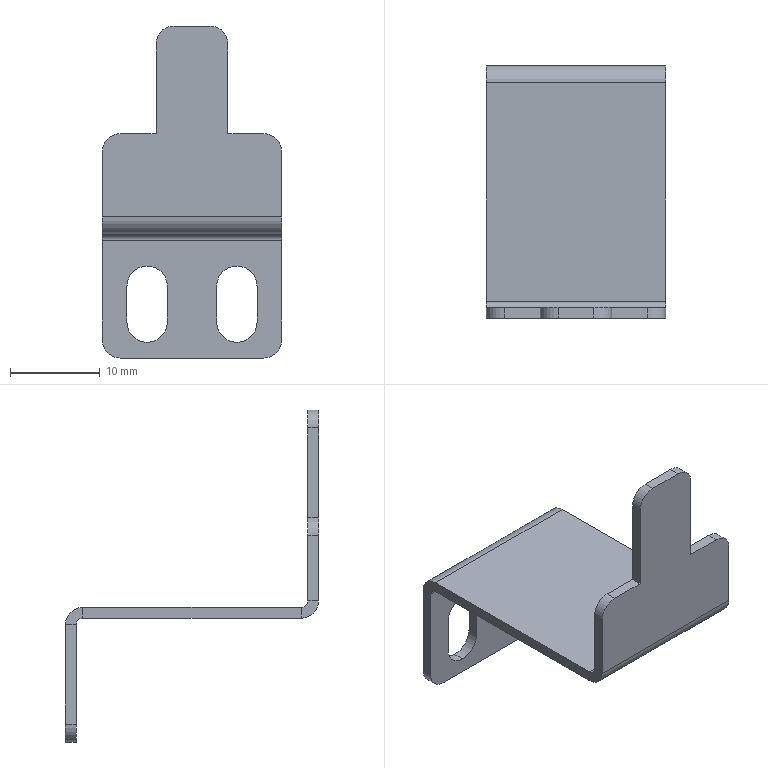Part | SolidWorks | features Cut 1, Fillet 1, FlatPattern 1, HoleWzd 1, SMBaseFlange 1, SheetMetal 1 | 1 solid | 42 faces | box 20 x 28.2 x 37 mm | volume 1248 mm3 | plane 26 | cylinder 16 | commonest cylinder face diameters 4 x6 4.5 x6 1.473 x2 3.873 x2
STEP:
#1=CARTESIAN_POINT('',(17.25,27.,-33.));
#2=VERTEX_POINT('',#1);
#3=CARTESIAN_POINT('',(15.,27.,-35.25));
#4=VERTEX_POINT('',#3);
#5=CARTESIAN_POINT('',(15.,27.,-33.));
#6=DIRECTION('',(0.,1.,0.));
#7=DIRECTION('',(0.,0.,1.));
#8=AXIS2_PLACEMENT_3D('',#5,#6,#7);
#9=CIRCLE('',#8,2.25);
#10=EDGE_CURVE('',#2,#4,#9,.T.);
#11=ORIENTED_EDGE('',*,*,#10,.T.);
#12=CARTESIAN_POINT('',(15.,25.8,-35.25));
#13=VERTEX_POINT('',#12);
#14=CARTESIAN_POINT('',(15.,25.8,-35.25));
#15=DIRECTION('',(0.,-1.,0.));
#16=VECTOR('',#15,1000.);
#17=LINE('',#14,#16);
#18=EDGE_CURVE('',#4,#13,#17,.T.);
#19=ORIENTED_EDGE('',*,*,#18,.T.);
#20=CARTESIAN_POINT('',(17.25,25.8,-33.));
#21=VERTEX_POINT('',#20);
#22=CARTESIAN_POINT('',(15.,25.8,-33.));
#23=DIRECTION('',(0.,-1.,0.));
#24=DIRECTION('',(0.,0.,-1.));
#25=AXIS2_PLACEMENT_3D('',#22,#23,#24);
#26=CIRCLE('',#25,2.25);
#27=EDGE_CURVE('',#13,#21,#26,.T.);
#28=ORIENTED_EDGE('',*,*,#27,.T.);
#29=CARTESIAN_POINT('',(17.25,40.8,-33.));
#30=DIRECTION('',(0.,1.,0.));
#31=VECTOR('',#30,1000.);
#32=LINE('',#29,#31);
#33=EDGE_CURVE('',#21,#2,#32,.T.);
#34=ORIENTED_EDGE('',*,*,#33,.T.);
#35=EDGE_LOOP('',(#11,#19,#28,#34));
#36=FACE_OUTER_BOUND('',#35,.T.);
#37=CARTESIAN_POINT('',(15.,25.8,-33.));
#38=DIRECTION('',(0.,-1.,0.));
#39=DIRECTION('',(0.,0.,-1.));
#40=AXIS2_PLACEMENT_3D('',#37,#38,#39);
#41=CYLINDRICAL_SURFACE('',#40,2.25);
#42=ADVANCED_FACE('',(#36),#41,.F.);
#43=CARTESIAN_POINT('',(7.25,27.,-33.));
#44=VERTEX_POINT('',#43);
#45=CARTESIAN_POINT('',(5.,27.,-35.25));
#46=VERTEX_POINT('',#45);
#47=CARTESIAN_POINT('',(5.,27.,-33.));
#48=DIRECTION('',(0.,1.,0.));
#49=DIRECTION('',(0.,0.,1.));
#50=AXIS2_PLACEMENT_3D('',#47,#48,#49);
#51=CIRCLE('',#50,2.25);
#52=EDGE_CURVE('',#44,#46,#51,.T.);
#53=ORIENTED_EDGE('',*,*,#52,.T.);
#54=CARTESIAN_POINT('',(5.,25.8,-35.25));
#55=VERTEX_POINT('',#54);
#56=CARTESIAN_POINT('',(5.,25.8,-35.25));
#57=DIRECTION('',(0.,-1.,0.));
#58=VECTOR('',#57,1000.);
#59=LINE('',#56,#58);
#60=EDGE_CURVE('',#46,#55,#59,.T.);
#61=ORIENTED_EDGE('',*,*,#60,.T.);
#62=CARTESIAN_POINT('',(7.25,25.8,-33.));
#63=VERTEX_POINT('',#62);
#64=CARTESIAN_POINT('',(5.,25.8,-33.));
#65=DIRECTION('',(0.,-1.,0.));
#66=DIRECTION('',(0.,0.,-1.));
#67=AXIS2_PLACEMENT_3D('',#64,#65,#66);
#68=CIRCLE('',#67,2.25);
#69=EDGE_CURVE('',#55,#63,#68,.T.);
#70=ORIENTED_EDGE('',*,*,#69,.T.);
#71=CARTESIAN_POINT('',(7.25,40.8,-33.));
#72=DIRECTION('',(0.,1.,0.));
#73=VECTOR('',#72,1000.);
#74=LINE('',#71,#73);
#75=EDGE_CURVE('',#63,#44,#74,.T.);
#76=ORIENTED_EDGE('',*,*,#75,.T.);
#77=EDGE_LOOP('',(#53,#61,#70,#76));
#78=FACE_OUTER_BOUND('',#77,.T.);
#79=CARTESIAN_POINT('',(5.,25.8,-33.));
#80=DIRECTION('',(0.,-1.,0.));
#81=DIRECTION('',(0.,0.,-1.));
#82=AXIS2_PLACEMENT_3D('',#79,#80,#81);
#83=CYLINDRICAL_SURFACE('',#82,2.25);
#84=ADVANCED_FACE('',(#78),#83,.F.);
#85=CARTESIAN_POINT('',(17.25,25.8,-29.));
#86=VERTEX_POINT('',#85);
#87=CARTESIAN_POINT('',(17.25,25.8,-29.));
#88=DIRECTION('',(0.,0.,-1.));
#89=VECTOR('',#88,1000.);
#90=LINE('',#87,#89);
#91=EDGE_CURVE('',#86,#21,#90,.T.);
#92=ORIENTED_EDGE('',*,*,#91,.T.);
#93=ORIENTED_EDGE('',*,*,#27,.F.);
#94=CARTESIAN_POINT('',(12.75,25.8,-33.));
#95=VERTEX_POINT('',#94);
#96=CARTESIAN_POINT('',(15.,25.8,-33.));
#97=DIRECTION('',(0.,-1.,0.));
#98=DIRECTION('',(0.,0.,-1.));
#99=AXIS2_PLACEMENT_3D('',#96,#97,#98);
#100=CIRCLE('',#99,2.25);
#101=EDGE_CURVE('',#95,#13,#100,.T.);
#102=ORIENTED_EDGE('',*,*,#101,.F.);
#103=CARTESIAN_POINT('',(12.75,25.8,-29.));
#104=VERTEX_POINT('',#103);
#105=CARTESIAN_POINT('',(12.75,25.8,-29.));
#106=DIRECTION('',(0.,0.,-1.));
#107=VECTOR('',#106,1000.);
#108=LINE('',#105,#107);
#109=EDGE_CURVE('',#104,#95,#108,.T.);
#110=ORIENTED_EDGE('',*,*,#109,.F.);
#111=CARTESIAN_POINT('',(15.,25.8,-29.));
#112=DIRECTION('',(0.,-1.,0.));
#113=DIRECTION('',(0.,0.,-1.));
#114=AXIS2_PLACEMENT_3D('',#111,#112,#113);
#115=CIRCLE('',#114,2.25);
#116=EDGE_CURVE('',#86,#104,#115,.T.);
#117=ORIENTED_EDGE('',*,*,#116,.F.);
#118=EDGE_LOOP('',(#92,#93,#102,#110,#117));
#119=FACE_BOUND('',#118,.T.);
#120=CARTESIAN_POINT('',(0.,25.8,-23.937));
#121=VERTEX_POINT('',#120);
#122=CARTESIAN_POINT('',(0.,25.8,-35.));
#123=VERTEX_POINT('',#122);
#124=CARTESIAN_POINT('',(0.,25.8,-22.));
#125=DIRECTION('',(0.,0.,-1.));
#126=VECTOR('',#125,1000.);
#127=LINE('',#124,#126);
#128=EDGE_CURVE('',#121,#123,#127,.T.);
#129=ORIENTED_EDGE('',*,*,#128,.T.);
#130=CARTESIAN_POINT('',(2.,25.8,-37.));
#131=VERTEX_POINT('',#130);
#132=CARTESIAN_POINT('',(2.,25.8,-35.));
#133=DIRECTION('',(0.,-1.,0.));
#134=DIRECTION('',(0.,0.,1.));
#135=AXIS2_PLACEMENT_3D('',#132,#133,#134);
#136=CIRCLE('',#135,2.);
#137=EDGE_CURVE('',#123,#131,#136,.T.);
#138=ORIENTED_EDGE('',*,*,#137,.T.);
#139=CARTESIAN_POINT('',(18.,25.8,-37.));
#140=VERTEX_POINT('',#139);
#141=CARTESIAN_POINT('',(20.,25.8,-37.));
#142=DIRECTION('',(-1.,0.,0.));
#143=VECTOR('',#142,1000.);
#144=LINE('',#141,#143);
#145=EDGE_CURVE('',#140,#131,#144,.T.);
#146=ORIENTED_EDGE('',*,*,#145,.F.);
#147=CARTESIAN_POINT('',(20.,25.8,-35.));
#148=VERTEX_POINT('',#147);
#149=CARTESIAN_POINT('',(18.,25.8,-35.));
#150=DIRECTION('',(0.,-1.,0.));
#151=DIRECTION('',(0.,0.,1.));
#152=AXIS2_PLACEMENT_3D('',#149,#150,#151);
#153=CIRCLE('',#152,2.);
#154=EDGE_CURVE('',#140,#148,#153,.T.);
#155=ORIENTED_EDGE('',*,*,#154,.T.);
#156=CARTESIAN_POINT('',(20.,25.8,-23.937));
#157=VERTEX_POINT('',#156);
#158=CARTESIAN_POINT('',(20.,25.8,-22.));
#159=DIRECTION('',(0.,0.,-1.));
#160=VECTOR('',#159,1000.);
#161=LINE('',#158,#160);
#162=EDGE_CURVE('',#157,#148,#161,.T.);
#163=ORIENTED_EDGE('',*,*,#162,.F.);
#164=CARTESIAN_POINT('',(20.,25.8,-23.937));
#165=DIRECTION('',(-1.,0.,0.));
#166=VECTOR('',#165,1000.);
#167=LINE('',#164,#166);
#168=EDGE_CURVE('',#157,#121,#167,.T.);
#169=ORIENTED_EDGE('',*,*,#168,.T.);
#170=EDGE_LOOP('',(#129,#138,#146,#155,#163,#169));
#171=FACE_OUTER_BOUND('',#170,.T.);
#172=CARTESIAN_POINT('',(7.25,25.8,-29.));
#173=VERTEX_POINT('',#172);
#174=CARTESIAN_POINT('',(7.25,25.8,-29.));
#175=DIRECTION('',(0.,0.,-1.));
#176=VECTOR('',#175,1000.);
#177=LINE('',#174,#176);
#178=EDGE_CURVE('',#173,#63,#177,.T.);
#179=ORIENTED_EDGE('',*,*,#178,.T.);
#180=ORIENTED_EDGE('',*,*,#69,.F.);
#181=CARTESIAN_POINT('',(2.75,25.8,-33.));
#182=VERTEX_POINT('',#181);
#183=CARTESIAN_POINT('',(5.,25.8,-33.));
#184=DIRECTION('',(0.,-1.,0.));
#185=DIRECTION('',(0.,0.,-1.));
#186=AXIS2_PLACEMENT_3D('',#183,#184,#185);
#187=CIRCLE('',#186,2.25);
#188=EDGE_CURVE('',#182,#55,#187,.T.);
#189=ORIENTED_EDGE('',*,*,#188,.F.);
#190=CARTESIAN_POINT('',(2.75,25.8,-29.));
#191=VERTEX_POINT('',#190);
#192=CARTESIAN_POINT('',(2.75,25.8,-29.));
#193=DIRECTION('',(0.,0.,-1.));
#194=VECTOR('',#193,1000.);
#195=LINE('',#192,#194);
#196=EDGE_CURVE('',#191,#182,#195,.T.);
#197=ORIENTED_EDGE('',*,*,#196,.F.);
#198=CARTESIAN_POINT('',(5.,25.8,-29.));
#199=DIRECTION('',(0.,-1.,0.));
#200=DIRECTION('',(0.,0.,-1.));
#201=AXIS2_PLACEMENT_3D('',#198,#199,#200);
#202=CIRCLE('',#201,2.25);
#203=EDGE_CURVE('',#173,#191,#202,.T.);
#204=ORIENTED_EDGE('',*,*,#203,.F.);
#205=EDGE_LOOP('',(#179,#180,#189,#197,#204));
#206=FACE_BOUND('',#205,.T.);
#207=CARTESIAN_POINT('',(20.,25.8,-22.));
#208=DIRECTION('',(0.,1.,0.));
#209=DIRECTION('',(0.,0.,1.));
#210=AXIS2_PLACEMENT_3D('',#207,#208,#209);
#211=PLANE('',#210);
#212=ADVANCED_FACE('',(#119,#171,#206),#211,.F.);
#213=CARTESIAN_POINT('',(20.,0.7366,-22.));
#214=VERTEX_POINT('',#213);
#215=CARTESIAN_POINT('',(20.,0.7366,-23.2));
#216=VERTEX_POINT('',#215);
#217=CARTESIAN_POINT('',(20.,0.7366,-22.));
#218=DIRECTION('',(0.,0.,-1.));
#219=VECTOR('',#218,1000.);
#220=LINE('',#217,#219);
#221=EDGE_CURVE('',#214,#216,#220,.T.);
#222=ORIENTED_EDGE('',*,*,#221,.F.);
#223=CARTESIAN_POINT('',(20.,0.,-21.263));
#224=VERTEX_POINT('',#223);
#225=CARTESIAN_POINT('',(20.,0.7366,-21.263));
#226=DIRECTION('',(1.,0.,0.));
#227=DIRECTION('',(0.,0.,1.));
#228=AXIS2_PLACEMENT_3D('',#225,#226,#227);
#229=CIRCLE('',#228,0.7366);
#230=EDGE_CURVE('',#224,#214,#229,.T.);
#231=ORIENTED_EDGE('',*,*,#230,.F.);
#232=CARTESIAN_POINT('',(20.,-1.2,-21.263));
#233=VERTEX_POINT('',#232);
#234=CARTESIAN_POINT('',(20.,-1.2,-21.263));
#235=DIRECTION('',(0.,1.,0.));
#236=VECTOR('',#235,1000.);
#237=LINE('',#234,#236);
#238=EDGE_CURVE('',#233,#224,#237,.T.);
#239=ORIENTED_EDGE('',*,*,#238,.F.);
#240=CARTESIAN_POINT('',(20.,0.7366,-21.263));
#241=DIRECTION('',(1.,0.,0.));
#242=DIRECTION('',(0.,0.,-1.));
#243=AXIS2_PLACEMENT_3D('',#240,#241,#242);
#244=CIRCLE('',#243,1.937);
#245=EDGE_CURVE('',#233,#216,#244,.T.);
#246=ORIENTED_EDGE('',*,*,#245,.T.);
#247=EDGE_LOOP('',(#222,#231,#239,#246));
#248=FACE_OUTER_BOUND('',#247,.T.);
#249=CARTESIAN_POINT('',(20.,0.7366,-22.));
#250=DIRECTION('',(1.,0.,0.));
#251=DIRECTION('',(0.,0.,-1.));
#252=AXIS2_PLACEMENT_3D('',#249,#250,#251);
#253=PLANE('',#252);
#254=ADVANCED_FACE('',(#248),#253,.T.);
#255=CARTESIAN_POINT('',(20.,25.063,-22.));
#256=VERTEX_POINT('',#255);
#257=CARTESIAN_POINT('',(20.,0.,-22.));
#258=DIRECTION('',(0.,1.,0.));
#259=VECTOR('',#258,1000.);
#260=LINE('',#257,#259);
#261=EDGE_CURVE('',#214,#256,#260,.T.);
#262=ORIENTED_EDGE('',*,*,#261,.F.);
#263=ORIENTED_EDGE('',*,*,#221,.T.);
#264=CARTESIAN_POINT('',(20.,25.063,-23.2));
#265=VERTEX_POINT('',#264);
#266=CARTESIAN_POINT('',(20.,0.,-23.2));
#267=DIRECTION('',(0.,1.,0.));
#268=VECTOR('',#267,1000.);
#269=LINE('',#266,#268);
#270=EDGE_CURVE('',#216,#265,#269,.T.);
#271=ORIENTED_EDGE('',*,*,#270,.T.);
#272=CARTESIAN_POINT('',(20.,25.063,-23.2));
#273=DIRECTION('',(0.,0.,1.));
#274=VECTOR('',#273,1000.);
#275=LINE('',#272,#274);
#276=EDGE_CURVE('',#265,#256,#275,.T.);
#277=ORIENTED_EDGE('',*,*,#276,.T.);
#278=EDGE_LOOP('',(#262,#263,#271,#277));
#279=FACE_OUTER_BOUND('',#278,.T.);
#280=CARTESIAN_POINT('',(20.,-1.2,-21.263));
#281=DIRECTION('',(1.,0.,0.));
#282=DIRECTION('',(0.,0.,-1.));
#283=AXIS2_PLACEMENT_3D('',#280,#281,#282);
#284=PLANE('',#283);
#285=ADVANCED_FACE('',(#279),#284,.T.);
#286=CARTESIAN_POINT('',(0.,0.,-21.263));
#287=VERTEX_POINT('',#286);
#288=CARTESIAN_POINT('',(0.,-1.2,-21.263));
#289=VERTEX_POINT('',#288);
#290=CARTESIAN_POINT('',(0.,0.,-21.263));
#291=DIRECTION('',(0.,-1.,0.));
#292=VECTOR('',#291,1000.);
#293=LINE('',#290,#292);
#294=EDGE_CURVE('',#287,#289,#293,.T.);
#295=ORIENTED_EDGE('',*,*,#294,.F.);
#296=CARTESIAN_POINT('',(0.,0.7366,-22.));
#297=VERTEX_POINT('',#296);
#298=CARTESIAN_POINT('',(0.,0.7366,-21.263));
#299=DIRECTION('',(1.,0.,0.));
#300=DIRECTION('',(0.,0.,1.));
#301=AXIS2_PLACEMENT_3D('',#298,#299,#300);
#302=CIRCLE('',#301,0.7366);
#303=EDGE_CURVE('',#287,#297,#302,.T.);
#304=ORIENTED_EDGE('',*,*,#303,.T.);
#305=CARTESIAN_POINT('',(0.,0.7366,-23.2));
#306=VERTEX_POINT('',#305);
#307=CARTESIAN_POINT('',(0.,0.7366,-23.2));
#308=DIRECTION('',(0.,0.,1.));
#309=VECTOR('',#308,1000.);
#310=LINE('',#307,#309);
#311=EDGE_CURVE('',#306,#297,#310,.T.);
#312=ORIENTED_EDGE('',*,*,#311,.F.);
#313=CARTESIAN_POINT('',(0.,0.7366,-21.263));
#314=DIRECTION('',(1.,0.,0.));
#315=DIRECTION('',(0.,0.,-1.));
#316=AXIS2_PLACEMENT_3D('',#313,#314,#315);
#317=CIRCLE('',#316,1.937);
#318=EDGE_CURVE('',#289,#306,#317,.T.);
#319=ORIENTED_EDGE('',*,*,#318,.F.);
#320=EDGE_LOOP('',(#295,#304,#312,#319));
#321=FACE_OUTER_BOUND('',#320,.T.);
#322=CARTESIAN_POINT('',(0.,0.,-21.263));
#323=DIRECTION('',(-1.,0.,0.));
#324=DIRECTION('',(0.,0.,1.));
#325=AXIS2_PLACEMENT_3D('',#322,#323,#324);
#326=PLANE('',#325);
#327=ADVANCED_FACE('',(#321),#326,.T.);
#328=CARTESIAN_POINT('',(0.,-1.2,-14.));
#329=VERTEX_POINT('',#328);
#330=CARTESIAN_POINT('',(0.,-1.2,0.));
#331=DIRECTION('',(0.,0.,-1.));
#332=VECTOR('',#331,1000.);
#333=LINE('',#330,#332);
#334=EDGE_CURVE('',#329,#289,#333,.T.);
#335=ORIENTED_EDGE('',*,*,#334,.F.);
#336=CARTESIAN_POINT('',(0.,0.,-14.));
#337=VERTEX_POINT('',#336);
#338=CARTESIAN_POINT('',(0.,0.,-14.));
#339=DIRECTION('',(0.,1.,0.));
#340=VECTOR('',#339,1000.);
#341=LINE('',#338,#340);
#342=EDGE_CURVE('',#329,#337,#341,.T.);
#343=ORIENTED_EDGE('',*,*,#342,.T.);
#344=CARTESIAN_POINT('',(0.,0.,0.));
#345=DIRECTION('',(0.,0.,-1.));
#346=VECTOR('',#345,1000.);
#347=LINE('',#344,#346);
#348=EDGE_CURVE('',#337,#287,#347,.T.);
#349=ORIENTED_EDGE('',*,*,#348,.T.);
#350=ORIENTED_EDGE('',*,*,#294,.T.);
#351=EDGE_LOOP('',(#335,#343,#349,#350));
#352=FACE_OUTER_BOUND('',#351,.T.);
#353=CARTESIAN_POINT('',(0.,0.7366,-23.2));
#354=DIRECTION('',(-1.,0.,0.));
#355=DIRECTION('',(0.,0.,1.));
#356=AXIS2_PLACEMENT_3D('',#353,#354,#355);
#357=PLANE('',#356);
#358=ADVANCED_FACE('',(#352),#357,.T.);
#359=CARTESIAN_POINT('',(20.,27.,-23.937));
#360=VERTEX_POINT('',#359);
#361=CARTESIAN_POINT('',(20.,27.,-23.937));
#362=DIRECTION('',(0.,-1.,0.));
#363=VECTOR('',#362,1000.);
#364=LINE('',#361,#363);
#365=EDGE_CURVE('',#360,#157,#364,.T.);
#366=ORIENTED_EDGE('',*,*,#365,.F.);
#367=CARTESIAN_POINT('',(20.,25.063,-23.937));
#368=DIRECTION('',(-1.,0.,0.));
#369=DIRECTION('',(0.,0.,-1.));
#370=AXIS2_PLACEMENT_3D('',#367,#368,#369);
#371=CIRCLE('',#370,1.937);
#372=EDGE_CURVE('',#256,#360,#371,.T.);
#373=ORIENTED_EDGE('',*,*,#372,.F.);
#374=ORIENTED_EDGE('',*,*,#276,.F.);
#375=CARTESIAN_POINT('',(20.,25.063,-23.937));
#376=DIRECTION('',(-1.,0.,0.));
#377=DIRECTION('',(0.,0.,-1.));
#378=AXIS2_PLACEMENT_3D('',#375,#376,#377);
#379=CIRCLE('',#378,0.7366);
#380=EDGE_CURVE('',#265,#157,#379,.T.);
#381=ORIENTED_EDGE('',*,*,#380,.T.);
#382=EDGE_LOOP('',(#366,#373,#374,#381));
#383=FACE_OUTER_BOUND('',#382,.T.);
#384=CARTESIAN_POINT('',(20.,27.,-23.937));
#385=DIRECTION('',(1.,0.,0.));
#386=DIRECTION('',(0.,0.,-1.));
#387=AXIS2_PLACEMENT_3D('',#384,#385,#386);
#388=PLANE('',#387);
#389=ADVANCED_FACE('',(#383),#388,.T.);
#390=ORIENTED_EDGE('',*,*,#162,.T.);
#391=CARTESIAN_POINT('',(20.,27.,-35.));
#392=VERTEX_POINT('',#391);
#393=CARTESIAN_POINT('',(20.,25.063,-35.));
#394=DIRECTION('',(0.,1.,0.));
#395=VECTOR('',#394,1000.);
#396=LINE('',#393,#395);
#397=EDGE_CURVE('',#148,#392,#396,.T.);
#398=ORIENTED_EDGE('',*,*,#397,.T.);
#399=CARTESIAN_POINT('',(20.,27.,-22.));
#400=DIRECTION('',(0.,0.,-1.));
#401=VECTOR('',#400,1000.);
#402=LINE('',#399,#401);
#403=EDGE_CURVE('',#360,#392,#402,.T.);
#404=ORIENTED_EDGE('',*,*,#403,.F.);
#405=ORIENTED_EDGE('',*,*,#365,.T.);
#406=EDGE_LOOP('',(#390,#398,#404,#405));
#407=FACE_OUTER_BOUND('',#406,.T.);
#408=CARTESIAN_POINT('',(20.,25.063,-23.2));
#409=DIRECTION('',(1.,0.,0.));
#410=DIRECTION('',(0.,0.,-1.));
#411=AXIS2_PLACEMENT_3D('',#408,#409,#410);
#412=PLANE('',#411);
#413=ADVANCED_FACE('',(#407),#412,.T.);
#414=CARTESIAN_POINT('',(0.,25.063,-22.));
#415=VERTEX_POINT('',#414);
#416=CARTESIAN_POINT('',(0.,25.063,-23.2));
#417=VERTEX_POINT('',#416);
#418=CARTESIAN_POINT('',(0.,25.063,-22.));
#419=DIRECTION('',(0.,0.,-1.));
#420=VECTOR('',#419,1000.);
#421=LINE('',#418,#420);
#422=EDGE_CURVE('',#415,#417,#421,.T.);
#423=ORIENTED_EDGE('',*,*,#422,.F.);
#424=CARTESIAN_POINT('',(0.,27.,-23.937));
#425=VERTEX_POINT('',#424);
#426=CARTESIAN_POINT('',(0.,25.063,-23.937));
#427=DIRECTION('',(-1.,0.,0.));
#428=DIRECTION('',(0.,0.,-1.));
#429=AXIS2_PLACEMENT_3D('',#426,#427,#428);
#430=CIRCLE('',#429,1.937);
#431=EDGE_CURVE('',#415,#425,#430,.T.);
#432=ORIENTED_EDGE('',*,*,#431,.T.);
#433=CARTESIAN_POINT('',(0.,25.8,-23.937));
#434=DIRECTION('',(0.,1.,0.));
#435=VECTOR('',#434,1000.);
#436=LINE('',#433,#435);
#437=EDGE_CURVE('',#121,#425,#436,.T.);
#438=ORIENTED_EDGE('',*,*,#437,.F.);
#439=CARTESIAN_POINT('',(0.,25.063,-23.937));
#440=DIRECTION('',(-1.,0.,0.));
#441=DIRECTION('',(0.,0.,-1.));
#442=AXIS2_PLACEMENT_3D('',#439,#440,#441);
#443=CIRCLE('',#442,0.7366);
#444=EDGE_CURVE('',#417,#121,#443,.T.);
#445=ORIENTED_EDGE('',*,*,#444,.F.);
#446=EDGE_LOOP('',(#423,#432,#438,#445));
#447=FACE_OUTER_BOUND('',#446,.T.);
#448=CARTESIAN_POINT('',(0.,25.063,-22.));
#449=DIRECTION('',(-1.,0.,0.));
#450=DIRECTION('',(0.,0.,1.));
#451=AXIS2_PLACEMENT_3D('',#448,#449,#450);
#452=PLANE('',#451);
#453=ADVANCED_FACE('',(#447),#452,.T.);
#454=CARTESIAN_POINT('',(0.,0.,-22.));
#455=DIRECTION('',(0.,1.,0.));
#456=VECTOR('',#455,1000.);
#457=LINE('',#454,#456);
#458=EDGE_CURVE('',#297,#415,#457,.T.);
#459=ORIENTED_EDGE('',*,*,#458,.T.);
#460=ORIENTED_EDGE('',*,*,#422,.T.);
#461=CARTESIAN_POINT('',(0.,0.,-23.2));
#462=DIRECTION('',(0.,1.,0.));
#463=VECTOR('',#462,1000.);
#464=LINE('',#461,#463);
#465=EDGE_CURVE('',#306,#417,#464,.T.);
#466=ORIENTED_EDGE('',*,*,#465,.F.);
#467=ORIENTED_EDGE('',*,*,#311,.T.);
#468=EDGE_LOOP('',(#459,#460,#466,#467));
#469=FACE_OUTER_BOUND('',#468,.T.);
#470=CARTESIAN_POINT('',(0.,25.8,-23.937));
#471=DIRECTION('',(-1.,0.,0.));
#472=DIRECTION('',(0.,0.,1.));
#473=AXIS2_PLACEMENT_3D('',#470,#471,#472);
#474=PLANE('',#473);
#475=ADVANCED_FACE('',(#469),#474,.T.);
#476=ORIENTED_EDGE('',*,*,#145,.T.);
#477=CARTESIAN_POINT('',(2.,27.,-37.));
#478=VERTEX_POINT('',#477);
#479=CARTESIAN_POINT('',(2.,27.,-37.));
#480=DIRECTION('',(0.,1.,0.));
#481=VECTOR('',#480,1000.);
#482=LINE('',#479,#481);
#483=EDGE_CURVE('',#131,#478,#482,.T.);
#484=ORIENTED_EDGE('',*,*,#483,.T.);
#485=CARTESIAN_POINT('',(18.,27.,-37.));
#486=VERTEX_POINT('',#485);
#487=CARTESIAN_POINT('',(20.,27.,-37.));
#488=DIRECTION('',(-1.,0.,0.));
#489=VECTOR('',#488,1000.);
#490=LINE('',#487,#489);
#491=EDGE_CURVE('',#486,#478,#490,.T.);
#492=ORIENTED_EDGE('',*,*,#491,.F.);
#493=CARTESIAN_POINT('',(18.,27.,-37.));
#494=DIRECTION('',(0.,-1.,0.));
#495=VECTOR('',#494,1000.);
#496=LINE('',#493,#495);
#497=EDGE_CURVE('',#486,#140,#496,.T.);
#498=ORIENTED_EDGE('',*,*,#497,.T.);
#499=EDGE_LOOP('',(#476,#484,#492,#498));
#500=FACE_OUTER_BOUND('',#499,.T.);
#501=CARTESIAN_POINT('',(20.,27.,-37.));
#502=DIRECTION('',(0.,0.,-1.));
#503=DIRECTION('',(-1.,0.,0.));
#504=AXIS2_PLACEMENT_3D('',#501,#502,#503);
#505=PLANE('',#504);
#506=ADVANCED_FACE('',(#500),#505,.T.);
#507=CARTESIAN_POINT('',(12.75,27.,-29.));
#508=VERTEX_POINT('',#507);
#509=CARTESIAN_POINT('',(17.25,27.,-29.));
#510=VERTEX_POINT('',#509);
#511=CARTESIAN_POINT('',(15.,27.,-29.));
#512=DIRECTION('',(0.,1.,0.));
#513=DIRECTION('',(0.,0.,1.));
#514=AXIS2_PLACEMENT_3D('',#511,#512,#513);
#515=CIRCLE('',#514,2.25);
#516=EDGE_CURVE('',#508,#510,#515,.T.);
#517=ORIENTED_EDGE('',*,*,#516,.F.);
#518=CARTESIAN_POINT('',(12.75,27.,-33.));
#519=VERTEX_POINT('',#518);
#520=CARTESIAN_POINT('',(12.75,27.,-22.));
#521=DIRECTION('',(0.,0.,1.));
#522=VECTOR('',#521,1000.);
#523=LINE('',#520,#522);
#524=EDGE_CURVE('',#519,#508,#523,.T.);
#525=ORIENTED_EDGE('',*,*,#524,.F.);
#526=CARTESIAN_POINT('',(15.,27.,-33.));
#527=DIRECTION('',(0.,1.,0.));
#528=DIRECTION('',(0.,0.,1.));
#529=AXIS2_PLACEMENT_3D('',#526,#527,#528);
#530=CIRCLE('',#529,2.25);
#531=EDGE_CURVE('',#4,#519,#530,.T.);
#532=ORIENTED_EDGE('',*,*,#531,.F.);
#533=ORIENTED_EDGE('',*,*,#10,.F.);
#534=CARTESIAN_POINT('',(17.25,27.,-22.));
#535=DIRECTION('',(0.,0.,1.));
#536=VECTOR('',#535,1000.);
#537=LINE('',#534,#536);
#538=EDGE_CURVE('',#2,#510,#537,.T.);
#539=ORIENTED_EDGE('',*,*,#538,.T.);
#540=EDGE_LOOP('',(#517,#525,#532,#533,#539));
#541=FACE_BOUND('',#540,.T.);
#542=CARTESIAN_POINT('',(2.75,27.,-29.));
#543=VERTEX_POINT('',#542);
#544=CARTESIAN_POINT('',(7.25,27.,-29.));
#545=VERTEX_POINT('',#544);
#546=CARTESIAN_POINT('',(5.,27.,-29.));
#547=DIRECTION('',(0.,1.,0.));
#548=DIRECTION('',(0.,0.,1.));
#549=AXIS2_PLACEMENT_3D('',#546,#547,#548);
#550=CIRCLE('',#549,2.25);
#551=EDGE_CURVE('',#543,#545,#550,.T.);
#552=ORIENTED_EDGE('',*,*,#551,.F.);
#553=CARTESIAN_POINT('',(2.75,27.,-33.));
#554=VERTEX_POINT('',#553);
#555=CARTESIAN_POINT('',(2.75,27.,-22.));
#556=DIRECTION('',(0.,0.,1.));
#557=VECTOR('',#556,1000.);
#558=LINE('',#555,#557);
#559=EDGE_CURVE('',#554,#543,#558,.T.);
#560=ORIENTED_EDGE('',*,*,#559,.F.);
#561=CARTESIAN_POINT('',(5.,27.,-33.));
#562=DIRECTION('',(0.,1.,0.));
#563=DIRECTION('',(0.,0.,1.));
#564=AXIS2_PLACEMENT_3D('',#561,#562,#563);
#565=CIRCLE('',#564,2.25);
#566=EDGE_CURVE('',#46,#554,#565,.T.);
#567=ORIENTED_EDGE('',*,*,#566,.F.);
#568=ORIENTED_EDGE('',*,*,#52,.F.);
#569=CARTESIAN_POINT('',(7.25,27.,-22.));
#570=DIRECTION('',(0.,0.,1.));
#571=VECTOR('',#570,1000.);
#572=LINE('',#569,#571);
#573=EDGE_CURVE('',#44,#545,#572,.T.);
#574=ORIENTED_EDGE('',*,*,#573,.T.);
#575=EDGE_LOOP('',(#552,#560,#567,#568,#574));
#576=FACE_BOUND('',#575,.T.);
#577=ORIENTED_EDGE('',*,*,#491,.T.);
#578=CARTESIAN_POINT('',(0.,27.,-35.));
#579=VERTEX_POINT('',#578);
#580=CARTESIAN_POINT('',(2.,27.,-35.));
#581=DIRECTION('',(0.,1.,0.));
#582=DIRECTION('',(0.,0.,1.));
#583=AXIS2_PLACEMENT_3D('',#580,#581,#582);
#584=CIRCLE('',#583,2.);
#585=EDGE_CURVE('',#478,#579,#584,.T.);
#586=ORIENTED_EDGE('',*,*,#585,.T.);
#587=CARTESIAN_POINT('',(0.,27.,-22.));
#588=DIRECTION('',(0.,0.,-1.));
#589=VECTOR('',#588,1000.);
#590=LINE('',#587,#589);
#591=EDGE_CURVE('',#425,#579,#590,.T.);
#592=ORIENTED_EDGE('',*,*,#591,.F.);
#593=CARTESIAN_POINT('',(20.,27.,-23.937));
#594=DIRECTION('',(-1.,0.,0.));
#595=VECTOR('',#594,1000.);
#596=LINE('',#593,#595);
#597=EDGE_CURVE('',#360,#425,#596,.T.);
#598=ORIENTED_EDGE('',*,*,#597,.F.);
#599=ORIENTED_EDGE('',*,*,#403,.T.);
#600=CARTESIAN_POINT('',(18.,27.,-35.));
#601=DIRECTION('',(0.,1.,0.));
#602=DIRECTION('',(0.,0.,1.));
#603=AXIS2_PLACEMENT_3D('',#600,#601,#602);
#604=CIRCLE('',#603,2.);
#605=EDGE_CURVE('',#392,#486,#604,.T.);
#606=ORIENTED_EDGE('',*,*,#605,.T.);
#607=EDGE_LOOP('',(#577,#586,#592,#598,#599,#606));
#608=FACE_OUTER_BOUND('',#607,.T.);
#609=CARTESIAN_POINT('',(20.,27.,-22.));
#610=DIRECTION('',(0.,1.,0.));
#611=DIRECTION('',(0.,0.,1.));
#612=AXIS2_PLACEMENT_3D('',#609,#610,#611);
#613=PLANE('',#612);
#614=ADVANCED_FACE('',(#541,#576,#608),#613,.T.);
#615=ORIENTED_EDGE('',*,*,#431,.F.);
#616=CARTESIAN_POINT('',(20.,25.063,-22.));
#617=DIRECTION('',(-1.,0.,0.));
#618=VECTOR('',#617,1000.);
#619=LINE('',#616,#618);
#620=EDGE_CURVE('',#256,#415,#619,.T.);
#621=ORIENTED_EDGE('',*,*,#620,.F.);
#622=ORIENTED_EDGE('',*,*,#372,.T.);
#623=ORIENTED_EDGE('',*,*,#597,.T.);
#624=EDGE_LOOP('',(#615,#621,#622,#623));
#625=FACE_OUTER_BOUND('',#624,.T.);
#626=CARTESIAN_POINT('',(20.,25.063,-23.937));
#627=DIRECTION('',(-1.,0.,0.));
#628=DIRECTION('',(0.,0.,1.));
#629=AXIS2_PLACEMENT_3D('',#626,#627,#628);
#630=CYLINDRICAL_SURFACE('',#629,1.937);
#631=ADVANCED_FACE('',(#625),#630,.T.);
#632=ORIENTED_EDGE('',*,*,#458,.F.);
#633=CARTESIAN_POINT('',(20.,0.7366,-22.));
#634=DIRECTION('',(-1.,0.,0.));
#635=VECTOR('',#634,1000.);
#636=LINE('',#633,#635);
#637=EDGE_CURVE('',#214,#297,#636,.T.);
#638=ORIENTED_EDGE('',*,*,#637,.F.);
#639=ORIENTED_EDGE('',*,*,#261,.T.);
#640=ORIENTED_EDGE('',*,*,#620,.T.);
#641=EDGE_LOOP('',(#632,#638,#639,#640));
#642=FACE_OUTER_BOUND('',#641,.T.);
#643=CARTESIAN_POINT('',(20.,0.,-22.));
#644=DIRECTION('',(0.,0.,1.));
#645=DIRECTION('',(1.,0.,0.));
#646=AXIS2_PLACEMENT_3D('',#643,#644,#645);
#647=PLANE('',#646);
#648=ADVANCED_FACE('',(#642),#647,.T.);
#649=ORIENTED_EDGE('',*,*,#303,.F.);
#650=CARTESIAN_POINT('',(20.,0.,-21.263));
#651=DIRECTION('',(-1.,0.,0.));
#652=VECTOR('',#651,1000.);
#653=LINE('',#650,#652);
#654=EDGE_CURVE('',#224,#287,#653,.T.);
#655=ORIENTED_EDGE('',*,*,#654,.F.);
#656=ORIENTED_EDGE('',*,*,#230,.T.);
#657=ORIENTED_EDGE('',*,*,#637,.T.);
#658=EDGE_LOOP('',(#649,#655,#656,#657));
#659=FACE_OUTER_BOUND('',#658,.T.);
#660=CARTESIAN_POINT('',(20.,0.7366,-21.263));
#661=DIRECTION('',(-1.,0.,0.));
#662=DIRECTION('',(0.,0.,1.));
#663=AXIS2_PLACEMENT_3D('',#660,#661,#662);
#664=CYLINDRICAL_SURFACE('',#663,0.7366);
#665=ADVANCED_FACE('',(#659),#664,.F.);
#666=CARTESIAN_POINT('',(6.,0.,-2.));
#667=VERTEX_POINT('',#666);
#668=CARTESIAN_POINT('',(6.,0.,-12.));
#669=VERTEX_POINT('',#668);
#670=CARTESIAN_POINT('',(6.,0.,0.));
#671=DIRECTION('',(0.,0.,-1.));
#672=VECTOR('',#671,1000.);
#673=LINE('',#670,#672);
#674=EDGE_CURVE('',#667,#669,#673,.T.);
#675=ORIENTED_EDGE('',*,*,#674,.F.);
#676=CARTESIAN_POINT('',(8.,0.,0.));
#677=VERTEX_POINT('',#676);
#678=CARTESIAN_POINT('',(8.,0.,-2.));
#679=DIRECTION('',(0.,1.,0.));
#680=DIRECTION('',(0.,0.,1.));
#681=AXIS2_PLACEMENT_3D('',#678,#679,#680);
#682=CIRCLE('',#681,2.);
#683=EDGE_CURVE('',#667,#677,#682,.T.);
#684=ORIENTED_EDGE('',*,*,#683,.T.);
#685=CARTESIAN_POINT('',(12.,0.,0.));
#686=VERTEX_POINT('',#685);
#687=CARTESIAN_POINT('',(20.,0.,0.));
#688=DIRECTION('',(-1.,0.,0.));
#689=VECTOR('',#688,1000.);
#690=LINE('',#687,#689);
#691=EDGE_CURVE('',#686,#677,#690,.T.);
#692=ORIENTED_EDGE('',*,*,#691,.F.);
#693=CARTESIAN_POINT('',(14.,0.,-2.));
#694=VERTEX_POINT('',#693);
#695=CARTESIAN_POINT('',(12.,0.,-2.));
#696=DIRECTION('',(0.,1.,0.));
#697=DIRECTION('',(0.,0.,1.));
#698=AXIS2_PLACEMENT_3D('',#695,#696,#697);
#699=CIRCLE('',#698,2.);
#700=EDGE_CURVE('',#686,#694,#699,.T.);
#701=ORIENTED_EDGE('',*,*,#700,.T.);
#702=CARTESIAN_POINT('',(14.,0.,-12.));
#703=VERTEX_POINT('',#702);
#704=CARTESIAN_POINT('',(14.,0.,0.));
#705=DIRECTION('',(0.,0.,1.));
#706=VECTOR('',#705,1000.);
#707=LINE('',#704,#706);
#708=EDGE_CURVE('',#703,#694,#707,.T.);
#709=ORIENTED_EDGE('',*,*,#708,.F.);
#710=CARTESIAN_POINT('',(18.,0.,-12.));
#711=VERTEX_POINT('',#710);
#712=CARTESIAN_POINT('',(20.,0.,-12.));
#713=DIRECTION('',(-1.,0.,0.));
#714=VECTOR('',#713,1000.);
#715=LINE('',#712,#714);
#716=EDGE_CURVE('',#711,#703,#715,.T.);
#717=ORIENTED_EDGE('',*,*,#716,.F.);
#718=CARTESIAN_POINT('',(20.,0.,-14.));
#719=VERTEX_POINT('',#718);
#720=CARTESIAN_POINT('',(18.,0.,-14.));
#721=DIRECTION('',(0.,1.,0.));
#722=DIRECTION('',(0.,0.,1.));
#723=AXIS2_PLACEMENT_3D('',#720,#721,#722);
#724=CIRCLE('',#723,2.);
#725=EDGE_CURVE('',#711,#719,#724,.T.);
#726=ORIENTED_EDGE('',*,*,#725,.T.);
#727=CARTESIAN_POINT('',(20.,0.,0.));
#728=DIRECTION('',(0.,0.,-1.));
#729=VECTOR('',#728,1000.);
#730=LINE('',#727,#729);
#731=EDGE_CURVE('',#719,#224,#730,.T.);
#732=ORIENTED_EDGE('',*,*,#731,.T.);
#733=ORIENTED_EDGE('',*,*,#654,.T.);
#734=ORIENTED_EDGE('',*,*,#348,.F.);
#735=CARTESIAN_POINT('',(2.,0.,-12.));
#736=VERTEX_POINT('',#735);
#737=CARTESIAN_POINT('',(2.,0.,-14.));
#738=DIRECTION('',(0.,1.,0.));
#739=DIRECTION('',(0.,0.,1.));
#740=AXIS2_PLACEMENT_3D('',#737,#738,#739);
#741=CIRCLE('',#740,2.);
#742=EDGE_CURVE('',#337,#736,#741,.T.);
#743=ORIENTED_EDGE('',*,*,#742,.T.);
#744=CARTESIAN_POINT('',(20.,0.,-12.));
#745=DIRECTION('',(-1.,0.,0.));
#746=VECTOR('',#745,1000.);
#747=LINE('',#744,#746);
#748=EDGE_CURVE('',#669,#736,#747,.T.);
#749=ORIENTED_EDGE('',*,*,#748,.F.);
#750=EDGE_LOOP('',(#675,#684,#692,#701,#709,#717,#726,#732,#733,#734,#743,#749));
#751=FACE_OUTER_BOUND('',#750,.T.);
#752=CARTESIAN_POINT('',(20.,0.,0.));
#753=DIRECTION('',(0.,1.,0.));
#754=DIRECTION('',(0.,0.,1.));
#755=AXIS2_PLACEMENT_3D('',#752,#753,#754);
#756=PLANE('',#755);
#757=ADVANCED_FACE('',(#751),#756,.T.);
#758=ORIENTED_EDGE('',*,*,#691,.T.);
#759=CARTESIAN_POINT('',(8.,-1.2,0.));
#760=VERTEX_POINT('',#759);
#761=CARTESIAN_POINT('',(8.,-1.2,0.));
#762=DIRECTION('',(0.,-1.,0.));
#763=VECTOR('',#762,1000.);
#764=LINE('',#761,#763);
#765=EDGE_CURVE('',#677,#760,#764,.T.);
#766=ORIENTED_EDGE('',*,*,#765,.T.);
#767=CARTESIAN_POINT('',(12.,-1.2,0.));
#768=VERTEX_POINT('',#767);
#769=CARTESIAN_POINT('',(20.,-1.2,0.));
#770=DIRECTION('',(-1.,0.,0.));
#771=VECTOR('',#770,1000.);
#772=LINE('',#769,#771);
#773=EDGE_CURVE('',#768,#760,#772,.T.);
#774=ORIENTED_EDGE('',*,*,#773,.F.);
#775=CARTESIAN_POINT('',(12.,0.,0.));
#776=DIRECTION('',(0.,1.,0.));
#777=VECTOR('',#776,1000.);
#778=LINE('',#775,#777);
#779=EDGE_CURVE('',#768,#686,#778,.T.);
#780=ORIENTED_EDGE('',*,*,#779,.T.);
#781=EDGE_LOOP('',(#758,#766,#774,#780));
#782=FACE_OUTER_BOUND('',#781,.T.);
#783=CARTESIAN_POINT('',(20.,-1.2,0.));
#784=DIRECTION('',(0.,0.,1.));
#785=DIRECTION('',(1.,0.,0.));
#786=AXIS2_PLACEMENT_3D('',#783,#784,#785);
#787=PLANE('',#786);
#788=ADVANCED_FACE('',(#782),#787,.T.);
#789=ORIENTED_EDGE('',*,*,#773,.T.);
#790=CARTESIAN_POINT('',(6.,-1.2,-2.));
#791=VERTEX_POINT('',#790);
#792=CARTESIAN_POINT('',(8.,-1.2,-2.));
#793=DIRECTION('',(0.,-1.,0.));
#794=DIRECTION('',(0.,0.,1.));
#795=AXIS2_PLACEMENT_3D('',#792,#793,#794);
#796=CIRCLE('',#795,2.);
#797=EDGE_CURVE('',#760,#791,#796,.T.);
#798=ORIENTED_EDGE('',*,*,#797,.T.);
#799=CARTESIAN_POINT('',(6.,-1.2,-12.));
#800=VERTEX_POINT('',#799);
#801=CARTESIAN_POINT('',(6.,-1.2,0.));
#802=DIRECTION('',(0.,0.,1.));
#803=VECTOR('',#802,1000.);
#804=LINE('',#801,#803);
#805=EDGE_CURVE('',#800,#791,#804,.T.);
#806=ORIENTED_EDGE('',*,*,#805,.F.);
#807=CARTESIAN_POINT('',(2.,-1.2,-12.));
#808=VERTEX_POINT('',#807);
#809=CARTESIAN_POINT('',(0.,-1.2,-12.));
#810=DIRECTION('',(1.,0.,0.));
#811=VECTOR('',#810,1000.);
#812=LINE('',#809,#811);
#813=EDGE_CURVE('',#808,#800,#812,.T.);
#814=ORIENTED_EDGE('',*,*,#813,.F.);
#815=CARTESIAN_POINT('',(2.,-1.2,-14.));
#816=DIRECTION('',(0.,-1.,0.));
#817=DIRECTION('',(0.,0.,1.));
#818=AXIS2_PLACEMENT_3D('',#815,#816,#817);
#819=CIRCLE('',#818,2.);
#820=EDGE_CURVE('',#808,#329,#819,.T.);
#821=ORIENTED_EDGE('',*,*,#820,.T.);
#822=ORIENTED_EDGE('',*,*,#334,.T.);
#823=CARTESIAN_POINT('',(20.,-1.2,-21.263));
#824=DIRECTION('',(-1.,0.,0.));
#825=VECTOR('',#824,1000.);
#826=LINE('',#823,#825);
#827=EDGE_CURVE('',#233,#289,#826,.T.);
#828=ORIENTED_EDGE('',*,*,#827,.F.);
#829=CARTESIAN_POINT('',(20.,-1.2,-14.));
#830=VERTEX_POINT('',#829);
#831=CARTESIAN_POINT('',(20.,-1.2,0.));
#832=DIRECTION('',(0.,0.,-1.));
#833=VECTOR('',#832,1000.);
#834=LINE('',#831,#833);
#835=EDGE_CURVE('',#830,#233,#834,.T.);
#836=ORIENTED_EDGE('',*,*,#835,.F.);
#837=CARTESIAN_POINT('',(18.,-1.2,-12.));
#838=VERTEX_POINT('',#837);
#839=CARTESIAN_POINT('',(18.,-1.2,-14.));
#840=DIRECTION('',(0.,-1.,0.));
#841=DIRECTION('',(0.,0.,1.));
#842=AXIS2_PLACEMENT_3D('',#839,#840,#841);
#843=CIRCLE('',#842,2.);
#844=EDGE_CURVE('',#830,#838,#843,.T.);
#845=ORIENTED_EDGE('',*,*,#844,.T.);
#846=CARTESIAN_POINT('',(14.,-1.2,-12.));
#847=VERTEX_POINT('',#846);
#848=CARTESIAN_POINT('',(20.,-1.2,-12.));
#849=DIRECTION('',(1.,0.,0.));
#850=VECTOR('',#849,1000.);
#851=LINE('',#848,#850);
#852=EDGE_CURVE('',#847,#838,#851,.T.);
#853=ORIENTED_EDGE('',*,*,#852,.F.);
#854=CARTESIAN_POINT('',(14.,-1.2,-2.));
#855=VERTEX_POINT('',#854);
#856=CARTESIAN_POINT('',(14.,-1.2,0.));
#857=DIRECTION('',(0.,0.,-1.));
#858=VECTOR('',#857,1000.);
#859=LINE('',#856,#858);
#860=EDGE_CURVE('',#855,#847,#859,.T.);
#861=ORIENTED_EDGE('',*,*,#860,.F.);
#862=CARTESIAN_POINT('',(12.,-1.2,-2.));
#863=DIRECTION('',(0.,-1.,0.));
#864=DIRECTION('',(0.,0.,1.));
#865=AXIS2_PLACEMENT_3D('',#862,#863,#864);
#866=CIRCLE('',#865,2.);
#867=EDGE_CURVE('',#855,#768,#866,.T.);
#868=ORIENTED_EDGE('',*,*,#867,.T.);
#869=EDGE_LOOP('',(#789,#798,#806,#814,#821,#822,#828,#836,#845,#853,#861,#868));
#870=FACE_OUTER_BOUND('',#869,.T.);
#871=CARTESIAN_POINT('',(20.,-1.2,0.));
#872=DIRECTION('',(0.,1.,0.));
#873=DIRECTION('',(0.,0.,1.));
#874=AXIS2_PLACEMENT_3D('',#871,#872,#873);
#875=PLANE('',#874);
#876=ADVANCED_FACE('',(#870),#875,.F.);
#877=ORIENTED_EDGE('',*,*,#318,.T.);
#878=CARTESIAN_POINT('',(20.,0.7366,-23.2));
#879=DIRECTION('',(-1.,0.,0.));
#880=VECTOR('',#879,1000.);
#881=LINE('',#878,#880);
#882=EDGE_CURVE('',#216,#306,#881,.T.);
#883=ORIENTED_EDGE('',*,*,#882,.F.);
#884=ORIENTED_EDGE('',*,*,#245,.F.);
#885=ORIENTED_EDGE('',*,*,#827,.T.);
#886=EDGE_LOOP('',(#877,#883,#884,#885));
#887=FACE_OUTER_BOUND('',#886,.T.);
#888=CARTESIAN_POINT('',(20.,0.7366,-21.263));
#889=DIRECTION('',(-1.,0.,0.));
#890=DIRECTION('',(0.,0.,1.));
#891=AXIS2_PLACEMENT_3D('',#888,#889,#890);
#892=CYLINDRICAL_SURFACE('',#891,1.937);
#893=ADVANCED_FACE('',(#887),#892,.T.);
#894=ORIENTED_EDGE('',*,*,#465,.T.);
#895=CARTESIAN_POINT('',(20.,25.063,-23.2));
#896=DIRECTION('',(-1.,0.,0.));
#897=VECTOR('',#896,1000.);
#898=LINE('',#895,#897);
#899=EDGE_CURVE('',#265,#417,#898,.T.);
#900=ORIENTED_EDGE('',*,*,#899,.F.);
#901=ORIENTED_EDGE('',*,*,#270,.F.);
#902=ORIENTED_EDGE('',*,*,#882,.T.);
#903=EDGE_LOOP('',(#894,#900,#901,#902));
#904=FACE_OUTER_BOUND('',#903,.T.);
#905=CARTESIAN_POINT('',(20.,0.,-23.2));
#906=DIRECTION('',(0.,0.,1.));
#907=DIRECTION('',(1.,0.,0.));
#908=AXIS2_PLACEMENT_3D('',#905,#906,#907);
#909=PLANE('',#908);
#910=ADVANCED_FACE('',(#904),#909,.F.);
#911=ORIENTED_EDGE('',*,*,#444,.T.);
#912=ORIENTED_EDGE('',*,*,#168,.F.);
#913=ORIENTED_EDGE('',*,*,#380,.F.);
#914=ORIENTED_EDGE('',*,*,#899,.T.);
#915=EDGE_LOOP('',(#911,#912,#913,#914));
#916=FACE_OUTER_BOUND('',#915,.T.);
#917=CARTESIAN_POINT('',(20.,25.063,-23.937));
#918=DIRECTION('',(-1.,0.,0.));
#919=DIRECTION('',(0.,0.,1.));
#920=AXIS2_PLACEMENT_3D('',#917,#918,#919);
#921=CYLINDRICAL_SURFACE('',#920,0.7366);
#922=ADVANCED_FACE('',(#916),#921,.F.);
#923=ORIENTED_EDGE('',*,*,#731,.F.);
#924=CARTESIAN_POINT('',(20.,-1.2,-14.));
#925=DIRECTION('',(0.,-1.,0.));
#926=VECTOR('',#925,1000.);
#927=LINE('',#924,#926);
#928=EDGE_CURVE('',#719,#830,#927,.T.);
#929=ORIENTED_EDGE('',*,*,#928,.T.);
#930=ORIENTED_EDGE('',*,*,#835,.T.);
#931=ORIENTED_EDGE('',*,*,#238,.T.);
#932=EDGE_LOOP('',(#923,#929,#930,#931));
#933=FACE_OUTER_BOUND('',#932,.T.);
#934=CARTESIAN_POINT('',(20.,25.063,-23.937));
#935=DIRECTION('',(1.,0.,0.));
#936=DIRECTION('',(0.,0.,-1.));
#937=AXIS2_PLACEMENT_3D('',#934,#935,#936);
#938=PLANE('',#937);
#939=ADVANCED_FACE('',(#933),#938,.T.);
#940=ORIENTED_EDGE('',*,*,#591,.T.);
#941=CARTESIAN_POINT('',(0.,25.8,-35.));
#942=DIRECTION('',(0.,-1.,0.));
#943=VECTOR('',#942,1000.);
#944=LINE('',#941,#943);
#945=EDGE_CURVE('',#579,#123,#944,.T.);
#946=ORIENTED_EDGE('',*,*,#945,.T.);
#947=ORIENTED_EDGE('',*,*,#128,.F.);
#948=ORIENTED_EDGE('',*,*,#437,.T.);
#949=EDGE_LOOP('',(#940,#946,#947,#948));
#950=FACE_OUTER_BOUND('',#949,.T.);
#951=CARTESIAN_POINT('',(0.,25.063,-23.937));
#952=DIRECTION('',(1.,0.,0.));
#953=DIRECTION('',(0.,0.,-1.));
#954=AXIS2_PLACEMENT_3D('',#951,#952,#953);
#955=PLANE('',#954);
#956=ADVANCED_FACE('',(#950),#955,.F.);
#957=ORIENTED_EDGE('',*,*,#852,.T.);
#958=CARTESIAN_POINT('',(18.,0.,-12.));
#959=DIRECTION('',(0.,1.,0.));
#960=VECTOR('',#959,1000.);
#961=LINE('',#958,#960);
#962=EDGE_CURVE('',#838,#711,#961,.T.);
#963=ORIENTED_EDGE('',*,*,#962,.T.);
#964=ORIENTED_EDGE('',*,*,#716,.T.);
#965=CARTESIAN_POINT('',(14.,27.,-12.));
#966=DIRECTION('',(0.,-1.,0.));
#967=VECTOR('',#966,1000.);
#968=LINE('',#965,#967);
#969=EDGE_CURVE('',#703,#847,#968,.T.);
#970=ORIENTED_EDGE('',*,*,#969,.T.);
#971=EDGE_LOOP('',(#957,#963,#964,#970));
#972=FACE_OUTER_BOUND('',#971,.T.);
#973=CARTESIAN_POINT('',(20.,27.,-12.));
#974=DIRECTION('',(0.,0.,-1.));
#975=DIRECTION('',(-1.,0.,0.));
#976=AXIS2_PLACEMENT_3D('',#973,#974,#975);
#977=PLANE('',#976);
#978=ADVANCED_FACE('',(#972),#977,.F.);
#979=ORIENTED_EDGE('',*,*,#708,.T.);
#980=CARTESIAN_POINT('',(14.,-1.2,-2.));
#981=DIRECTION('',(0.,-1.,0.));
#982=VECTOR('',#981,1000.);
#983=LINE('',#980,#982);
#984=EDGE_CURVE('',#694,#855,#983,.T.);
#985=ORIENTED_EDGE('',*,*,#984,.T.);
#986=ORIENTED_EDGE('',*,*,#860,.T.);
#987=ORIENTED_EDGE('',*,*,#969,.F.);
#988=EDGE_LOOP('',(#979,#985,#986,#987));
#989=FACE_OUTER_BOUND('',#988,.T.);
#990=CARTESIAN_POINT('',(14.,27.,0.));
#991=DIRECTION('',(-1.,0.,0.));
#992=DIRECTION('',(0.,0.,1.));
#993=AXIS2_PLACEMENT_3D('',#990,#991,#992);
#994=PLANE('',#993);
#995=ADVANCED_FACE('',(#989),#994,.F.);
#996=ORIENTED_EDGE('',*,*,#805,.T.);
#997=CARTESIAN_POINT('',(6.,0.,-2.));
#998=DIRECTION('',(0.,1.,0.));
#999=VECTOR('',#998,1000.);
#1000=LINE('',#997,#999);
#1001=EDGE_CURVE('',#791,#667,#1000,.T.);
#1002=ORIENTED_EDGE('',*,*,#1001,.T.);
#1003=ORIENTED_EDGE('',*,*,#674,.T.);
#1004=CARTESIAN_POINT('',(6.,27.,-12.));
#1005=DIRECTION('',(0.,-1.,0.));
#1006=VECTOR('',#1005,1000.);
#1007=LINE('',#1004,#1006);
#1008=EDGE_CURVE('',#669,#800,#1007,.T.);
#1009=ORIENTED_EDGE('',*,*,#1008,.T.);
#1010=EDGE_LOOP('',(#996,#1002,#1003,#1009));
#1011=FACE_OUTER_BOUND('',#1010,.T.);
#1012=CARTESIAN_POINT('',(6.,27.,0.));
#1013=DIRECTION('',(1.,0.,0.));
#1014=DIRECTION('',(0.,0.,-1.));
#1015=AXIS2_PLACEMENT_3D('',#1012,#1013,#1014);
#1016=PLANE('',#1015);
#1017=ADVANCED_FACE('',(#1011),#1016,.F.);
#1018=ORIENTED_EDGE('',*,*,#748,.T.);
#1019=CARTESIAN_POINT('',(2.,-1.2,-12.));
#1020=DIRECTION('',(0.,-1.,0.));
#1021=VECTOR('',#1020,1000.);
#1022=LINE('',#1019,#1021);
#1023=EDGE_CURVE('',#736,#808,#1022,.T.);
#1024=ORIENTED_EDGE('',*,*,#1023,.T.);
#1025=ORIENTED_EDGE('',*,*,#813,.T.);
#1026=ORIENTED_EDGE('',*,*,#1008,.F.);
#1027=EDGE_LOOP('',(#1018,#1024,#1025,#1026));
#1028=FACE_OUTER_BOUND('',#1027,.T.);
#1029=CARTESIAN_POINT('',(0.,27.,-12.));
#1030=DIRECTION('',(0.,0.,-1.));
#1031=DIRECTION('',(-1.,0.,0.));
#1032=AXIS2_PLACEMENT_3D('',#1029,#1030,#1031);
#1033=PLANE('',#1032);
#1034=ADVANCED_FACE('',(#1028),#1033,.F.);
#1035=ORIENTED_EDGE('',*,*,#60,.F.);
#1036=ORIENTED_EDGE('',*,*,#566,.T.);
#1037=CARTESIAN_POINT('',(2.75,25.8,-33.));
#1038=DIRECTION('',(0.,1.,0.));
#1039=VECTOR('',#1038,1000.);
#1040=LINE('',#1037,#1039);
#1041=EDGE_CURVE('',#182,#554,#1040,.T.);
#1042=ORIENTED_EDGE('',*,*,#1041,.F.);
#1043=ORIENTED_EDGE('',*,*,#188,.T.);
#1044=EDGE_LOOP('',(#1035,#1036,#1042,#1043));
#1045=FACE_OUTER_BOUND('',#1044,.T.);
#1046=CARTESIAN_POINT('',(5.,25.8,-33.));
#1047=DIRECTION('',(0.,-1.,0.));
#1048=DIRECTION('',(0.,0.,-1.));
#1049=AXIS2_PLACEMENT_3D('',#1046,#1047,#1048);
#1050=CYLINDRICAL_SURFACE('',#1049,2.25);
#1051=ADVANCED_FACE('',(#1045),#1050,.F.);
#1052=ORIENTED_EDGE('',*,*,#551,.T.);
#1053=CARTESIAN_POINT('',(7.25,40.8,-29.));
#1054=DIRECTION('',(0.,1.,0.));
#1055=VECTOR('',#1054,1000.);
#1056=LINE('',#1053,#1055);
#1057=EDGE_CURVE('',#173,#545,#1056,.T.);
#1058=ORIENTED_EDGE('',*,*,#1057,.F.);
#1059=ORIENTED_EDGE('',*,*,#203,.T.);
#1060=CARTESIAN_POINT('',(2.75,25.8,-29.));
#1061=DIRECTION('',(0.,-1.,0.));
#1062=VECTOR('',#1061,1000.);
#1063=LINE('',#1060,#1062);
#1064=EDGE_CURVE('',#543,#191,#1063,.T.);
#1065=ORIENTED_EDGE('',*,*,#1064,.F.);
#1066=EDGE_LOOP('',(#1052,#1058,#1059,#1065));
#1067=FACE_OUTER_BOUND('',#1066,.T.);
#1068=CARTESIAN_POINT('',(5.,25.8,-29.));
#1069=DIRECTION('',(0.,-1.,0.));
#1070=DIRECTION('',(0.,0.,-1.));
#1071=AXIS2_PLACEMENT_3D('',#1068,#1069,#1070);
#1072=CYLINDRICAL_SURFACE('',#1071,2.25);
#1073=ADVANCED_FACE('',(#1067),#1072,.F.);
#1074=ORIENTED_EDGE('',*,*,#75,.F.);
#1075=ORIENTED_EDGE('',*,*,#178,.F.);
#1076=ORIENTED_EDGE('',*,*,#1057,.T.);
#1077=ORIENTED_EDGE('',*,*,#573,.F.);
#1078=EDGE_LOOP('',(#1074,#1075,#1076,#1077));
#1079=FACE_OUTER_BOUND('',#1078,.T.);
#1080=CARTESIAN_POINT('',(7.25,40.8,-29.));
#1081=DIRECTION('',(-1.,0.,0.));
#1082=DIRECTION('',(0.,-1.,0.));
#1083=AXIS2_PLACEMENT_3D('',#1080,#1081,#1082);
#1084=PLANE('',#1083);
#1085=ADVANCED_FACE('',(#1079),#1084,.T.);
#1086=ORIENTED_EDGE('',*,*,#559,.T.);
#1087=ORIENTED_EDGE('',*,*,#1064,.T.);
#1088=ORIENTED_EDGE('',*,*,#196,.T.);
#1089=ORIENTED_EDGE('',*,*,#1041,.T.);
#1090=EDGE_LOOP('',(#1086,#1087,#1088,#1089));
#1091=FACE_OUTER_BOUND('',#1090,.T.);
#1092=CARTESIAN_POINT('',(2.75,25.8,-29.));
#1093=DIRECTION('',(-1.,0.,0.));
#1094=DIRECTION('',(0.,0.,1.));
#1095=AXIS2_PLACEMENT_3D('',#1092,#1093,#1094);
#1096=PLANE('',#1095);
#1097=ADVANCED_FACE('',(#1091),#1096,.F.);
#1098=ORIENTED_EDGE('',*,*,#18,.F.);
#1099=ORIENTED_EDGE('',*,*,#531,.T.);
#1100=CARTESIAN_POINT('',(12.75,25.8,-33.));
#1101=DIRECTION('',(0.,1.,0.));
#1102=VECTOR('',#1101,1000.);
#1103=LINE('',#1100,#1102);
#1104=EDGE_CURVE('',#95,#519,#1103,.T.);
#1105=ORIENTED_EDGE('',*,*,#1104,.F.);
#1106=ORIENTED_EDGE('',*,*,#101,.T.);
#1107=EDGE_LOOP('',(#1098,#1099,#1105,#1106));
#1108=FACE_OUTER_BOUND('',#1107,.T.);
#1109=CARTESIAN_POINT('',(15.,25.8,-33.));
#1110=DIRECTION('',(0.,-1.,0.));
#1111=DIRECTION('',(0.,0.,-1.));
#1112=AXIS2_PLACEMENT_3D('',#1109,#1110,#1111);
#1113=CYLINDRICAL_SURFACE('',#1112,2.25);
#1114=ADVANCED_FACE('',(#1108),#1113,.F.);
#1115=ORIENTED_EDGE('',*,*,#516,.T.);
#1116=CARTESIAN_POINT('',(17.25,40.8,-29.));
#1117=DIRECTION('',(0.,1.,0.));
#1118=VECTOR('',#1117,1000.);
#1119=LINE('',#1116,#1118);
#1120=EDGE_CURVE('',#86,#510,#1119,.T.);
#1121=ORIENTED_EDGE('',*,*,#1120,.F.);
#1122=ORIENTED_EDGE('',*,*,#116,.T.);
#1123=CARTESIAN_POINT('',(12.75,25.8,-29.));
#1124=DIRECTION('',(0.,-1.,0.));
#1125=VECTOR('',#1124,1000.);
#1126=LINE('',#1123,#1125);
#1127=EDGE_CURVE('',#508,#104,#1126,.T.);
#1128=ORIENTED_EDGE('',*,*,#1127,.F.);
#1129=EDGE_LOOP('',(#1115,#1121,#1122,#1128));
#1130=FACE_OUTER_BOUND('',#1129,.T.);
#1131=CARTESIAN_POINT('',(15.,25.8,-29.));
#1132=DIRECTION('',(0.,-1.,0.));
#1133=DIRECTION('',(0.,0.,-1.));
#1134=AXIS2_PLACEMENT_3D('',#1131,#1132,#1133);
#1135=CYLINDRICAL_SURFACE('',#1134,2.25);
#1136=ADVANCED_FACE('',(#1130),#1135,.F.);
#1137=ORIENTED_EDGE('',*,*,#33,.F.);
#1138=ORIENTED_EDGE('',*,*,#91,.F.);
#1139=ORIENTED_EDGE('',*,*,#1120,.T.);
#1140=ORIENTED_EDGE('',*,*,#538,.F.);
#1141=EDGE_LOOP('',(#1137,#1138,#1139,#1140));
#1142=FACE_OUTER_BOUND('',#1141,.T.);
#1143=CARTESIAN_POINT('',(17.25,40.8,-29.));
#1144=DIRECTION('',(-1.,0.,0.));
#1145=DIRECTION('',(0.,-1.,0.));
#1146=AXIS2_PLACEMENT_3D('',#1143,#1144,#1145);
#1147=PLANE('',#1146);
#1148=ADVANCED_FACE('',(#1142),#1147,.T.);
#1149=ORIENTED_EDGE('',*,*,#524,.T.);
#1150=ORIENTED_EDGE('',*,*,#1127,.T.);
#1151=ORIENTED_EDGE('',*,*,#109,.T.);
#1152=ORIENTED_EDGE('',*,*,#1104,.T.);
#1153=EDGE_LOOP('',(#1149,#1150,#1151,#1152));
#1154=FACE_OUTER_BOUND('',#1153,.T.);
#1155=CARTESIAN_POINT('',(12.75,25.8,-29.));
#1156=DIRECTION('',(-1.,0.,0.));
#1157=DIRECTION('',(0.,0.,1.));
#1158=AXIS2_PLACEMENT_3D('',#1155,#1156,#1157);
#1159=PLANE('',#1158);
#1160=ADVANCED_FACE('',(#1154),#1159,.F.);
#1161=ORIENTED_EDGE('',*,*,#683,.F.);
#1162=ORIENTED_EDGE('',*,*,#1001,.F.);
#1163=ORIENTED_EDGE('',*,*,#797,.F.);
#1164=ORIENTED_EDGE('',*,*,#765,.F.);
#1165=EDGE_LOOP('',(#1161,#1162,#1163,#1164));
#1166=FACE_OUTER_BOUND('',#1165,.T.);
#1167=CARTESIAN_POINT('',(8.,-1.2,-2.));
#1168=DIRECTION('',(0.,1.,0.));
#1169=DIRECTION('',(0.,0.,1.));
#1170=AXIS2_PLACEMENT_3D('',#1167,#1168,#1169);
#1171=CYLINDRICAL_SURFACE('',#1170,2.);
#1172=ADVANCED_FACE('',(#1166),#1171,.T.);
#1173=ORIENTED_EDGE('',*,*,#700,.F.);
#1174=ORIENTED_EDGE('',*,*,#779,.F.);
#1175=ORIENTED_EDGE('',*,*,#867,.F.);
#1176=ORIENTED_EDGE('',*,*,#984,.F.);
#1177=EDGE_LOOP('',(#1173,#1174,#1175,#1176));
#1178=FACE_OUTER_BOUND('',#1177,.T.);
#1179=CARTESIAN_POINT('',(12.,27.,-2.));
#1180=DIRECTION('',(0.,1.,0.));
#1181=DIRECTION('',(0.,0.,1.));
#1182=AXIS2_PLACEMENT_3D('',#1179,#1180,#1181);
#1183=CYLINDRICAL_SURFACE('',#1182,2.);
#1184=ADVANCED_FACE('',(#1178),#1183,.T.);
#1185=ORIENTED_EDGE('',*,*,#844,.F.);
#1186=ORIENTED_EDGE('',*,*,#928,.F.);
#1187=ORIENTED_EDGE('',*,*,#725,.F.);
#1188=ORIENTED_EDGE('',*,*,#962,.F.);
#1189=EDGE_LOOP('',(#1185,#1186,#1187,#1188));
#1190=FACE_OUTER_BOUND('',#1189,.T.);
#1191=CARTESIAN_POINT('',(18.,27.,-14.));
#1192=DIRECTION('',(0.,-1.,0.));
#1193=DIRECTION('',(0.,0.,-1.));
#1194=AXIS2_PLACEMENT_3D('',#1191,#1192,#1193);
#1195=CYLINDRICAL_SURFACE('',#1194,2.);
#1196=ADVANCED_FACE('',(#1190),#1195,.T.);
#1197=ORIENTED_EDGE('',*,*,#742,.F.);
#1198=ORIENTED_EDGE('',*,*,#342,.F.);
#1199=ORIENTED_EDGE('',*,*,#820,.F.);
#1200=ORIENTED_EDGE('',*,*,#1023,.F.);
#1201=EDGE_LOOP('',(#1197,#1198,#1199,#1200));
#1202=FACE_OUTER_BOUND('',#1201,.T.);
#1203=CARTESIAN_POINT('',(2.,27.,-14.));
#1204=DIRECTION('',(0.,1.,0.));
#1205=DIRECTION('',(0.,0.,1.));
#1206=AXIS2_PLACEMENT_3D('',#1203,#1204,#1205);
#1207=CYLINDRICAL_SURFACE('',#1206,2.);
#1208=ADVANCED_FACE('',(#1202),#1207,.T.);
#1209=ORIENTED_EDGE('',*,*,#585,.F.);
#1210=ORIENTED_EDGE('',*,*,#483,.F.);
#1211=ORIENTED_EDGE('',*,*,#137,.F.);
#1212=ORIENTED_EDGE('',*,*,#945,.F.);
#1213=EDGE_LOOP('',(#1209,#1210,#1211,#1212));
#1214=FACE_OUTER_BOUND('',#1213,.T.);
#1215=CARTESIAN_POINT('',(2.,25.063,-35.));
#1216=DIRECTION('',(0.,1.,0.));
#1217=DIRECTION('',(0.,0.,1.));
#1218=AXIS2_PLACEMENT_3D('',#1215,#1216,#1217);
#1219=CYLINDRICAL_SURFACE('',#1218,2.);
#1220=ADVANCED_FACE('',(#1214),#1219,.T.);
#1221=ORIENTED_EDGE('',*,*,#605,.F.);
#1222=ORIENTED_EDGE('',*,*,#397,.F.);
#1223=ORIENTED_EDGE('',*,*,#154,.F.);
#1224=ORIENTED_EDGE('',*,*,#497,.F.);
#1225=EDGE_LOOP('',(#1221,#1222,#1223,#1224));
#1226=FACE_OUTER_BOUND('',#1225,.T.);
#1227=CARTESIAN_POINT('',(18.,27.,-35.));
#1228=DIRECTION('',(0.,-1.,0.));
#1229=DIRECTION('',(0.,0.,-1.));
#1230=AXIS2_PLACEMENT_3D('',#1227,#1228,#1229);
#1231=CYLINDRICAL_SURFACE('',#1230,2.);
#1232=ADVANCED_FACE('',(#1226),#1231,.T.);
#1233=CLOSED_SHELL('',(#42,#84,#212,#254,#285,#327,#358,#389,#413,#453,#475,#506,#614,#631,#648,#665,#757,#788,#876,#893,#910,#922,#939,#956,#978,#995,#1017,#1034,#1051,#1073,#1085,#1097,#1114,#1136,#1148,#1160,#1172,#1184,#1196,#1208,#1220,#1232));
#1234=MANIFOLD_SOLID_BREP('',#1233);
#1235=CARTESIAN_POINT('',(0.,0.,0.));
#1236=DIRECTION('',(0.,0.,1.));
#1237=DIRECTION('',(1.,0.,0.));
#1238=AXIS2_PLACEMENT_3D('',#1235,#1236,#1237);
#1239=(LENGTH_UNIT()NAMED_UNIT(*)SI_UNIT(.MILLI.,.METRE.));
#1240=UNCERTAINTY_MEASURE_WITH_UNIT(LENGTH_MEASURE(0.00001),#1239,'','');
#1241=(NAMED_UNIT(*)PLANE_ANGLE_UNIT()SI_UNIT($,.RADIAN.));
#1242=(NAMED_UNIT(*)SI_UNIT($,.STERADIAN.)SOLID_ANGLE_UNIT());
#1243=(GEOMETRIC_REPRESENTATION_CONTEXT(3)GLOBAL_UNCERTAINTY_ASSIGNED_CONTEXT((#1240))GLOBAL_UNIT_ASSIGNED_CONTEXT((#1239,#1241,#1242))REPRESENTATION_CONTEXT('',''));
#1244=ADVANCED_BREP_SHAPE_REPRESENTATION('',(#1234,#1238),#1243);